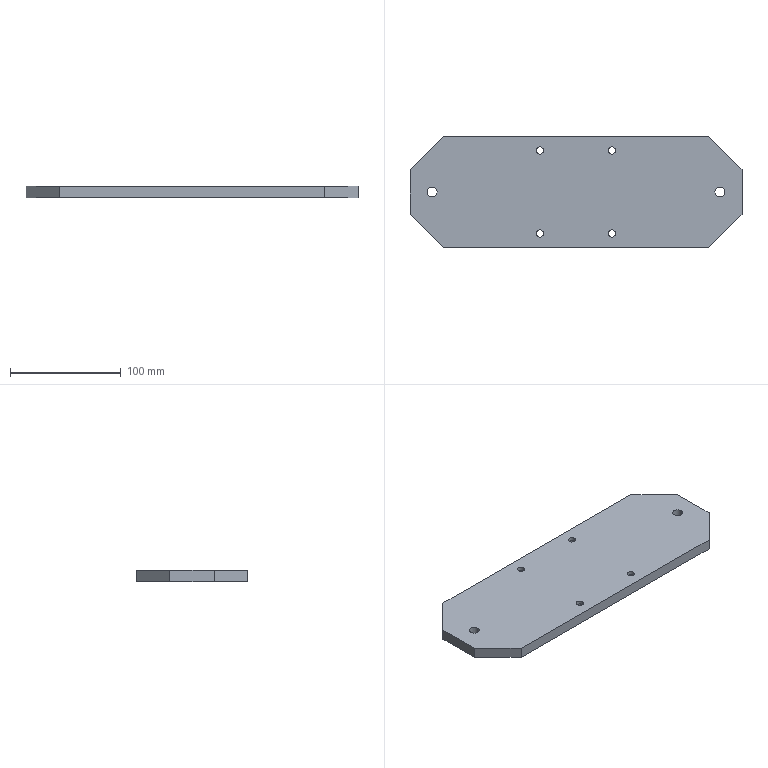Part | SolidWorks | features HoleWzd 2, Chamfer 1, Extrusion 1 | 1 solid | 34 faces | box 300 x 100 x 10 mm | volume 277705 mm3 | cylinder 20 | plane 14 | commonest cylinder face diameters 6.6 x8 11 x8 9 x4
STEP:
#1=CARTESIAN_POINT('',(125.5,0.,10.));
#2=VERTEX_POINT('',#1);
#3=CARTESIAN_POINT('',(134.5,0.,10.));
#4=VERTEX_POINT('',#3);
#5=CARTESIAN_POINT('',(130.,0.,10.));
#6=DIRECTION('',(0.,0.,1.));
#7=DIRECTION('',(1.,0.,0.));
#8=AXIS2_PLACEMENT_3D('',#5,#6,#7);
#9=CIRCLE('',#8,4.5);
#10=EDGE_CURVE('',#2,#4,#9,.T.);
#11=ORIENTED_EDGE('',*,*,#10,.T.);
#12=CARTESIAN_POINT('',(134.5,0.,0.));
#13=VERTEX_POINT('',#12);
#14=CARTESIAN_POINT('',(134.5,0.,0.));
#15=DIRECTION('',(0.,0.,-1.));
#16=VECTOR('',#15,1000.);
#17=LINE('',#14,#16);
#18=EDGE_CURVE('',#4,#13,#17,.T.);
#19=ORIENTED_EDGE('',*,*,#18,.T.);
#20=CARTESIAN_POINT('',(125.5,0.,0.));
#21=VERTEX_POINT('',#20);
#22=CARTESIAN_POINT('',(130.,0.,0.));
#23=DIRECTION('',(0.,0.,-1.));
#24=DIRECTION('',(-1.,0.,0.));
#25=AXIS2_PLACEMENT_3D('',#22,#23,#24);
#26=CIRCLE('',#25,4.5);
#27=EDGE_CURVE('',#13,#21,#26,.T.);
#28=ORIENTED_EDGE('',*,*,#27,.T.);
#29=CARTESIAN_POINT('',(125.5,0.,0.));
#30=DIRECTION('',(0.,0.,-1.));
#31=VECTOR('',#30,1000.);
#32=LINE('',#29,#31);
#33=EDGE_CURVE('',#2,#21,#32,.T.);
#34=ORIENTED_EDGE('',*,*,#33,.F.);
#35=EDGE_LOOP('',(#11,#19,#28,#34));
#36=FACE_OUTER_BOUND('',#35,.T.);
#37=CARTESIAN_POINT('',(130.,0.,0.));
#38=DIRECTION('',(0.,0.,-1.));
#39=DIRECTION('',(-1.,0.,0.));
#40=AXIS2_PLACEMENT_3D('',#37,#38,#39);
#41=CYLINDRICAL_SURFACE('',#40,4.5);
#42=ADVANCED_FACE('',(#36),#41,.F.);
#43=CARTESIAN_POINT('',(-134.5,0.,10.));
#44=VERTEX_POINT('',#43);
#45=CARTESIAN_POINT('',(-125.5,0.,10.));
#46=VERTEX_POINT('',#45);
#47=CARTESIAN_POINT('',(-130.,0.,10.));
#48=DIRECTION('',(0.,0.,1.));
#49=DIRECTION('',(1.,0.,0.));
#50=AXIS2_PLACEMENT_3D('',#47,#48,#49);
#51=CIRCLE('',#50,4.5);
#52=EDGE_CURVE('',#44,#46,#51,.T.);
#53=ORIENTED_EDGE('',*,*,#52,.T.);
#54=CARTESIAN_POINT('',(-125.5,0.,0.));
#55=VERTEX_POINT('',#54);
#56=CARTESIAN_POINT('',(-125.5,0.,0.));
#57=DIRECTION('',(0.,0.,-1.));
#58=VECTOR('',#57,1000.);
#59=LINE('',#56,#58);
#60=EDGE_CURVE('',#46,#55,#59,.T.);
#61=ORIENTED_EDGE('',*,*,#60,.T.);
#62=CARTESIAN_POINT('',(-134.5,0.,0.));
#63=VERTEX_POINT('',#62);
#64=CARTESIAN_POINT('',(-130.,0.,0.));
#65=DIRECTION('',(0.,0.,-1.));
#66=DIRECTION('',(-1.,0.,0.));
#67=AXIS2_PLACEMENT_3D('',#64,#65,#66);
#68=CIRCLE('',#67,4.5);
#69=EDGE_CURVE('',#55,#63,#68,.T.);
#70=ORIENTED_EDGE('',*,*,#69,.T.);
#71=CARTESIAN_POINT('',(-134.5,0.,0.));
#72=DIRECTION('',(0.,0.,-1.));
#73=VECTOR('',#72,1000.);
#74=LINE('',#71,#73);
#75=EDGE_CURVE('',#44,#63,#74,.T.);
#76=ORIENTED_EDGE('',*,*,#75,.F.);
#77=EDGE_LOOP('',(#53,#61,#70,#76));
#78=FACE_OUTER_BOUND('',#77,.T.);
#79=CARTESIAN_POINT('',(-130.,0.,0.));
#80=DIRECTION('',(0.,0.,-1.));
#81=DIRECTION('',(-1.,0.,0.));
#82=AXIS2_PLACEMENT_3D('',#79,#80,#81);
#83=CYLINDRICAL_SURFACE('',#82,4.5);
#84=ADVANCED_FACE('',(#78),#83,.F.);
#85=CARTESIAN_POINT('',(-27.1,-37.5,6.8));
#86=VERTEX_POINT('',#85);
#87=CARTESIAN_POINT('',(-38.1,-37.5,6.8));
#88=VERTEX_POINT('',#87);
#89=CARTESIAN_POINT('',(-32.6,-37.5,6.8));
#90=DIRECTION('',(0.,0.,-1.));
#91=DIRECTION('',(-1.,0.,0.));
#92=AXIS2_PLACEMENT_3D('',#89,#90,#91);
#93=CIRCLE('',#92,5.5);
#94=EDGE_CURVE('',#86,#88,#93,.T.);
#95=ORIENTED_EDGE('',*,*,#94,.F.);
#96=CARTESIAN_POINT('',(-27.1,-37.5,0.));
#97=VERTEX_POINT('',#96);
#98=CARTESIAN_POINT('',(-27.1,-37.5,0.));
#99=DIRECTION('',(0.,0.,-1.));
#100=VECTOR('',#99,1000.);
#101=LINE('',#98,#100);
#102=EDGE_CURVE('',#86,#97,#101,.T.);
#103=ORIENTED_EDGE('',*,*,#102,.T.);
#104=CARTESIAN_POINT('',(-38.1,-37.5,0.));
#105=VERTEX_POINT('',#104);
#106=CARTESIAN_POINT('',(-32.6,-37.5,0.));
#107=DIRECTION('',(0.,0.,-1.));
#108=DIRECTION('',(-1.,0.,0.));
#109=AXIS2_PLACEMENT_3D('',#106,#107,#108);
#110=CIRCLE('',#109,5.5);
#111=EDGE_CURVE('',#97,#105,#110,.T.);
#112=ORIENTED_EDGE('',*,*,#111,.T.);
#113=CARTESIAN_POINT('',(-38.1,-37.5,0.));
#114=DIRECTION('',(0.,0.,-1.));
#115=VECTOR('',#114,1000.);
#116=LINE('',#113,#115);
#117=EDGE_CURVE('',#88,#105,#116,.T.);
#118=ORIENTED_EDGE('',*,*,#117,.F.);
#119=EDGE_LOOP('',(#95,#103,#112,#118));
#120=FACE_OUTER_BOUND('',#119,.T.);
#121=CARTESIAN_POINT('',(-32.6,-37.5,0.));
#122=DIRECTION('',(0.,0.,-1.));
#123=DIRECTION('',(-1.,0.,0.));
#124=AXIS2_PLACEMENT_3D('',#121,#122,#123);
#125=CYLINDRICAL_SURFACE('',#124,5.5);
#126=ADVANCED_FACE('',(#120),#125,.F.);
#127=CARTESIAN_POINT('',(-35.9,-37.5,10.));
#128=VERTEX_POINT('',#127);
#129=CARTESIAN_POINT('',(-29.3,-37.5,10.));
#130=VERTEX_POINT('',#129);
#131=CARTESIAN_POINT('',(-32.6,-37.5,10.));
#132=DIRECTION('',(0.,0.,1.));
#133=DIRECTION('',(1.,0.,0.));
#134=AXIS2_PLACEMENT_3D('',#131,#132,#133);
#135=CIRCLE('',#134,3.3);
#136=EDGE_CURVE('',#128,#130,#135,.T.);
#137=ORIENTED_EDGE('',*,*,#136,.T.);
#138=CARTESIAN_POINT('',(-29.3,-37.5,6.8));
#139=VERTEX_POINT('',#138);
#140=CARTESIAN_POINT('',(-29.3,-37.5,0.));
#141=DIRECTION('',(0.,0.,-1.));
#142=VECTOR('',#141,1000.);
#143=LINE('',#140,#142);
#144=EDGE_CURVE('',#130,#139,#143,.T.);
#145=ORIENTED_EDGE('',*,*,#144,.T.);
#146=CARTESIAN_POINT('',(-35.9,-37.5,6.8));
#147=VERTEX_POINT('',#146);
#148=CARTESIAN_POINT('',(-32.6,-37.5,6.8));
#149=DIRECTION('',(0.,0.,-1.));
#150=DIRECTION('',(-1.,0.,0.));
#151=AXIS2_PLACEMENT_3D('',#148,#149,#150);
#152=CIRCLE('',#151,3.3);
#153=EDGE_CURVE('',#139,#147,#152,.T.);
#154=ORIENTED_EDGE('',*,*,#153,.T.);
#155=CARTESIAN_POINT('',(-35.9,-37.5,0.));
#156=DIRECTION('',(0.,0.,-1.));
#157=VECTOR('',#156,1000.);
#158=LINE('',#155,#157);
#159=EDGE_CURVE('',#128,#147,#158,.T.);
#160=ORIENTED_EDGE('',*,*,#159,.F.);
#161=EDGE_LOOP('',(#137,#145,#154,#160));
#162=FACE_OUTER_BOUND('',#161,.T.);
#163=CARTESIAN_POINT('',(-32.6,-37.5,0.));
#164=DIRECTION('',(0.,0.,-1.));
#165=DIRECTION('',(-1.,0.,0.));
#166=AXIS2_PLACEMENT_3D('',#163,#164,#165);
#167=CYLINDRICAL_SURFACE('',#166,3.3);
#168=ADVANCED_FACE('',(#162),#167,.F.);
#169=CARTESIAN_POINT('',(37.9,-37.5,6.8));
#170=VERTEX_POINT('',#169);
#171=CARTESIAN_POINT('',(26.9,-37.5,6.8));
#172=VERTEX_POINT('',#171);
#173=CARTESIAN_POINT('',(32.4,-37.5,6.8));
#174=DIRECTION('',(0.,0.,-1.));
#175=DIRECTION('',(-1.,0.,0.));
#176=AXIS2_PLACEMENT_3D('',#173,#174,#175);
#177=CIRCLE('',#176,5.5);
#178=EDGE_CURVE('',#170,#172,#177,.T.);
#179=ORIENTED_EDGE('',*,*,#178,.F.);
#180=CARTESIAN_POINT('',(37.9,-37.5,0.));
#181=VERTEX_POINT('',#180);
#182=CARTESIAN_POINT('',(37.9,-37.5,0.));
#183=DIRECTION('',(0.,0.,-1.));
#184=VECTOR('',#183,1000.);
#185=LINE('',#182,#184);
#186=EDGE_CURVE('',#170,#181,#185,.T.);
#187=ORIENTED_EDGE('',*,*,#186,.T.);
#188=CARTESIAN_POINT('',(26.9,-37.5,0.));
#189=VERTEX_POINT('',#188);
#190=CARTESIAN_POINT('',(32.4,-37.5,0.));
#191=DIRECTION('',(0.,0.,-1.));
#192=DIRECTION('',(-1.,0.,0.));
#193=AXIS2_PLACEMENT_3D('',#190,#191,#192);
#194=CIRCLE('',#193,5.5);
#195=EDGE_CURVE('',#181,#189,#194,.T.);
#196=ORIENTED_EDGE('',*,*,#195,.T.);
#197=CARTESIAN_POINT('',(26.9,-37.5,0.));
#198=DIRECTION('',(0.,0.,-1.));
#199=VECTOR('',#198,1000.);
#200=LINE('',#197,#199);
#201=EDGE_CURVE('',#172,#189,#200,.T.);
#202=ORIENTED_EDGE('',*,*,#201,.F.);
#203=EDGE_LOOP('',(#179,#187,#196,#202));
#204=FACE_OUTER_BOUND('',#203,.T.);
#205=CARTESIAN_POINT('',(32.4,-37.5,0.));
#206=DIRECTION('',(0.,0.,-1.));
#207=DIRECTION('',(-1.,0.,0.));
#208=AXIS2_PLACEMENT_3D('',#205,#206,#207);
#209=CYLINDRICAL_SURFACE('',#208,5.5);
#210=ADVANCED_FACE('',(#204),#209,.F.);
#211=CARTESIAN_POINT('',(29.1,-37.5,10.));
#212=VERTEX_POINT('',#211);
#213=CARTESIAN_POINT('',(35.7,-37.5,10.));
#214=VERTEX_POINT('',#213);
#215=CARTESIAN_POINT('',(32.4,-37.5,10.));
#216=DIRECTION('',(0.,0.,1.));
#217=DIRECTION('',(1.,0.,0.));
#218=AXIS2_PLACEMENT_3D('',#215,#216,#217);
#219=CIRCLE('',#218,3.3);
#220=EDGE_CURVE('',#212,#214,#219,.T.);
#221=ORIENTED_EDGE('',*,*,#220,.T.);
#222=CARTESIAN_POINT('',(35.7,-37.5,6.8));
#223=VERTEX_POINT('',#222);
#224=CARTESIAN_POINT('',(35.7,-37.5,0.));
#225=DIRECTION('',(0.,0.,-1.));
#226=VECTOR('',#225,1000.);
#227=LINE('',#224,#226);
#228=EDGE_CURVE('',#214,#223,#227,.T.);
#229=ORIENTED_EDGE('',*,*,#228,.T.);
#230=CARTESIAN_POINT('',(29.1,-37.5,6.8));
#231=VERTEX_POINT('',#230);
#232=CARTESIAN_POINT('',(32.4,-37.5,6.8));
#233=DIRECTION('',(0.,0.,-1.));
#234=DIRECTION('',(-1.,0.,0.));
#235=AXIS2_PLACEMENT_3D('',#232,#233,#234);
#236=CIRCLE('',#235,3.3);
#237=EDGE_CURVE('',#223,#231,#236,.T.);
#238=ORIENTED_EDGE('',*,*,#237,.T.);
#239=CARTESIAN_POINT('',(29.1,-37.5,0.));
#240=DIRECTION('',(0.,0.,-1.));
#241=VECTOR('',#240,1000.);
#242=LINE('',#239,#241);
#243=EDGE_CURVE('',#212,#231,#242,.T.);
#244=ORIENTED_EDGE('',*,*,#243,.F.);
#245=EDGE_LOOP('',(#221,#229,#238,#244));
#246=FACE_OUTER_BOUND('',#245,.T.);
#247=CARTESIAN_POINT('',(32.4,-37.5,0.));
#248=DIRECTION('',(0.,0.,-1.));
#249=DIRECTION('',(-1.,0.,0.));
#250=AXIS2_PLACEMENT_3D('',#247,#248,#249);
#251=CYLINDRICAL_SURFACE('',#250,3.3);
#252=ADVANCED_FACE('',(#246),#251,.F.);
#253=CARTESIAN_POINT('',(37.9,37.5,6.8));
#254=VERTEX_POINT('',#253);
#255=CARTESIAN_POINT('',(26.9,37.5,6.8));
#256=VERTEX_POINT('',#255);
#257=CARTESIAN_POINT('',(32.4,37.5,6.8));
#258=DIRECTION('',(0.,0.,-1.));
#259=DIRECTION('',(-1.,0.,0.));
#260=AXIS2_PLACEMENT_3D('',#257,#258,#259);
#261=CIRCLE('',#260,5.5);
#262=EDGE_CURVE('',#254,#256,#261,.T.);
#263=ORIENTED_EDGE('',*,*,#262,.F.);
#264=CARTESIAN_POINT('',(37.9,37.5,0.));
#265=VERTEX_POINT('',#264);
#266=CARTESIAN_POINT('',(37.9,37.5,0.));
#267=DIRECTION('',(0.,0.,-1.));
#268=VECTOR('',#267,1000.);
#269=LINE('',#266,#268);
#270=EDGE_CURVE('',#254,#265,#269,.T.);
#271=ORIENTED_EDGE('',*,*,#270,.T.);
#272=CARTESIAN_POINT('',(26.9,37.5,0.));
#273=VERTEX_POINT('',#272);
#274=CARTESIAN_POINT('',(32.4,37.5,0.));
#275=DIRECTION('',(0.,0.,-1.));
#276=DIRECTION('',(-1.,0.,0.));
#277=AXIS2_PLACEMENT_3D('',#274,#275,#276);
#278=CIRCLE('',#277,5.5);
#279=EDGE_CURVE('',#265,#273,#278,.T.);
#280=ORIENTED_EDGE('',*,*,#279,.T.);
#281=CARTESIAN_POINT('',(26.9,37.5,0.));
#282=DIRECTION('',(0.,0.,-1.));
#283=VECTOR('',#282,1000.);
#284=LINE('',#281,#283);
#285=EDGE_CURVE('',#256,#273,#284,.T.);
#286=ORIENTED_EDGE('',*,*,#285,.F.);
#287=EDGE_LOOP('',(#263,#271,#280,#286));
#288=FACE_OUTER_BOUND('',#287,.T.);
#289=CARTESIAN_POINT('',(32.4,37.5,0.));
#290=DIRECTION('',(0.,0.,-1.));
#291=DIRECTION('',(-1.,0.,0.));
#292=AXIS2_PLACEMENT_3D('',#289,#290,#291);
#293=CYLINDRICAL_SURFACE('',#292,5.5);
#294=ADVANCED_FACE('',(#288),#293,.F.);
#295=CARTESIAN_POINT('',(29.1,37.5,10.));
#296=VERTEX_POINT('',#295);
#297=CARTESIAN_POINT('',(35.7,37.5,10.));
#298=VERTEX_POINT('',#297);
#299=CARTESIAN_POINT('',(32.4,37.5,10.));
#300=DIRECTION('',(0.,0.,1.));
#301=DIRECTION('',(1.,0.,0.));
#302=AXIS2_PLACEMENT_3D('',#299,#300,#301);
#303=CIRCLE('',#302,3.3);
#304=EDGE_CURVE('',#296,#298,#303,.T.);
#305=ORIENTED_EDGE('',*,*,#304,.T.);
#306=CARTESIAN_POINT('',(35.7,37.5,6.8));
#307=VERTEX_POINT('',#306);
#308=CARTESIAN_POINT('',(35.7,37.5,0.));
#309=DIRECTION('',(0.,0.,-1.));
#310=VECTOR('',#309,1000.);
#311=LINE('',#308,#310);
#312=EDGE_CURVE('',#298,#307,#311,.T.);
#313=ORIENTED_EDGE('',*,*,#312,.T.);
#314=CARTESIAN_POINT('',(29.1,37.5,6.8));
#315=VERTEX_POINT('',#314);
#316=CARTESIAN_POINT('',(32.4,37.5,6.8));
#317=DIRECTION('',(0.,0.,-1.));
#318=DIRECTION('',(-1.,0.,0.));
#319=AXIS2_PLACEMENT_3D('',#316,#317,#318);
#320=CIRCLE('',#319,3.3);
#321=EDGE_CURVE('',#307,#315,#320,.T.);
#322=ORIENTED_EDGE('',*,*,#321,.T.);
#323=CARTESIAN_POINT('',(29.1,37.5,0.));
#324=DIRECTION('',(0.,0.,-1.));
#325=VECTOR('',#324,1000.);
#326=LINE('',#323,#325);
#327=EDGE_CURVE('',#296,#315,#326,.T.);
#328=ORIENTED_EDGE('',*,*,#327,.F.);
#329=EDGE_LOOP('',(#305,#313,#322,#328));
#330=FACE_OUTER_BOUND('',#329,.T.);
#331=CARTESIAN_POINT('',(32.4,37.5,0.));
#332=DIRECTION('',(0.,0.,-1.));
#333=DIRECTION('',(-1.,0.,0.));
#334=AXIS2_PLACEMENT_3D('',#331,#332,#333);
#335=CYLINDRICAL_SURFACE('',#334,3.3);
#336=ADVANCED_FACE('',(#330),#335,.F.);
#337=CARTESIAN_POINT('',(-27.1,37.5,6.8));
#338=VERTEX_POINT('',#337);
#339=CARTESIAN_POINT('',(-38.1,37.5,6.8));
#340=VERTEX_POINT('',#339);
#341=CARTESIAN_POINT('',(-32.6,37.5,6.8));
#342=DIRECTION('',(0.,0.,-1.));
#343=DIRECTION('',(-1.,0.,0.));
#344=AXIS2_PLACEMENT_3D('',#341,#342,#343);
#345=CIRCLE('',#344,5.5);
#346=EDGE_CURVE('',#338,#340,#345,.T.);
#347=ORIENTED_EDGE('',*,*,#346,.F.);
#348=CARTESIAN_POINT('',(-27.1,37.5,0.));
#349=VERTEX_POINT('',#348);
#350=CARTESIAN_POINT('',(-27.1,37.5,0.));
#351=DIRECTION('',(0.,0.,-1.));
#352=VECTOR('',#351,1000.);
#353=LINE('',#350,#352);
#354=EDGE_CURVE('',#338,#349,#353,.T.);
#355=ORIENTED_EDGE('',*,*,#354,.T.);
#356=CARTESIAN_POINT('',(-38.1,37.5,0.));
#357=VERTEX_POINT('',#356);
#358=CARTESIAN_POINT('',(-32.6,37.5,0.));
#359=DIRECTION('',(0.,0.,-1.));
#360=DIRECTION('',(-1.,0.,0.));
#361=AXIS2_PLACEMENT_3D('',#358,#359,#360);
#362=CIRCLE('',#361,5.5);
#363=EDGE_CURVE('',#349,#357,#362,.T.);
#364=ORIENTED_EDGE('',*,*,#363,.T.);
#365=CARTESIAN_POINT('',(-38.1,37.5,0.));
#366=DIRECTION('',(0.,0.,-1.));
#367=VECTOR('',#366,1000.);
#368=LINE('',#365,#367);
#369=EDGE_CURVE('',#340,#357,#368,.T.);
#370=ORIENTED_EDGE('',*,*,#369,.F.);
#371=EDGE_LOOP('',(#347,#355,#364,#370));
#372=FACE_OUTER_BOUND('',#371,.T.);
#373=CARTESIAN_POINT('',(-32.6,37.5,0.));
#374=DIRECTION('',(0.,0.,-1.));
#375=DIRECTION('',(-1.,0.,0.));
#376=AXIS2_PLACEMENT_3D('',#373,#374,#375);
#377=CYLINDRICAL_SURFACE('',#376,5.5);
#378=ADVANCED_FACE('',(#372),#377,.F.);
#379=CARTESIAN_POINT('',(-35.9,37.5,10.));
#380=VERTEX_POINT('',#379);
#381=CARTESIAN_POINT('',(-29.3,37.5,10.));
#382=VERTEX_POINT('',#381);
#383=CARTESIAN_POINT('',(-32.6,37.5,10.));
#384=DIRECTION('',(0.,0.,1.));
#385=DIRECTION('',(1.,0.,0.));
#386=AXIS2_PLACEMENT_3D('',#383,#384,#385);
#387=CIRCLE('',#386,3.3);
#388=EDGE_CURVE('',#380,#382,#387,.T.);
#389=ORIENTED_EDGE('',*,*,#388,.T.);
#390=CARTESIAN_POINT('',(-29.3,37.5,6.8));
#391=VERTEX_POINT('',#390);
#392=CARTESIAN_POINT('',(-29.3,37.5,0.));
#393=DIRECTION('',(0.,0.,-1.));
#394=VECTOR('',#393,1000.);
#395=LINE('',#392,#394);
#396=EDGE_CURVE('',#382,#391,#395,.T.);
#397=ORIENTED_EDGE('',*,*,#396,.T.);
#398=CARTESIAN_POINT('',(-35.9,37.5,6.8));
#399=VERTEX_POINT('',#398);
#400=CARTESIAN_POINT('',(-32.6,37.5,6.8));
#401=DIRECTION('',(0.,0.,-1.));
#402=DIRECTION('',(-1.,0.,0.));
#403=AXIS2_PLACEMENT_3D('',#400,#401,#402);
#404=CIRCLE('',#403,3.3);
#405=EDGE_CURVE('',#391,#399,#404,.T.);
#406=ORIENTED_EDGE('',*,*,#405,.T.);
#407=CARTESIAN_POINT('',(-35.9,37.5,0.));
#408=DIRECTION('',(0.,0.,-1.));
#409=VECTOR('',#408,1000.);
#410=LINE('',#407,#409);
#411=EDGE_CURVE('',#380,#399,#410,.T.);
#412=ORIENTED_EDGE('',*,*,#411,.F.);
#413=EDGE_LOOP('',(#389,#397,#406,#412));
#414=FACE_OUTER_BOUND('',#413,.T.);
#415=CARTESIAN_POINT('',(-32.6,37.5,0.));
#416=DIRECTION('',(0.,0.,-1.));
#417=DIRECTION('',(-1.,0.,0.));
#418=AXIS2_PLACEMENT_3D('',#415,#416,#417);
#419=CYLINDRICAL_SURFACE('',#418,3.3);
#420=ADVANCED_FACE('',(#414),#419,.F.);
#421=CARTESIAN_POINT('',(130.,0.,0.));
#422=DIRECTION('',(0.,0.,-1.));
#423=DIRECTION('',(-1.,0.,0.));
#424=AXIS2_PLACEMENT_3D('',#421,#422,#423);
#425=CIRCLE('',#424,4.5);
#426=EDGE_CURVE('',#21,#13,#425,.T.);
#427=ORIENTED_EDGE('',*,*,#426,.F.);
#428=ORIENTED_EDGE('',*,*,#27,.F.);
#429=EDGE_LOOP('',(#427,#428));
#430=FACE_BOUND('',#429,.T.);
#431=CARTESIAN_POINT('',(-32.6,-37.5,0.));
#432=DIRECTION('',(0.,0.,-1.));
#433=DIRECTION('',(-1.,0.,0.));
#434=AXIS2_PLACEMENT_3D('',#431,#432,#433);
#435=CIRCLE('',#434,5.5);
#436=EDGE_CURVE('',#105,#97,#435,.T.);
#437=ORIENTED_EDGE('',*,*,#436,.F.);
#438=ORIENTED_EDGE('',*,*,#111,.F.);
#439=EDGE_LOOP('',(#437,#438));
#440=FACE_BOUND('',#439,.T.);
#441=CARTESIAN_POINT('',(32.4,-37.5,0.));
#442=DIRECTION('',(0.,0.,-1.));
#443=DIRECTION('',(-1.,0.,0.));
#444=AXIS2_PLACEMENT_3D('',#441,#442,#443);
#445=CIRCLE('',#444,5.5);
#446=EDGE_CURVE('',#189,#181,#445,.T.);
#447=ORIENTED_EDGE('',*,*,#446,.F.);
#448=ORIENTED_EDGE('',*,*,#195,.F.);
#449=EDGE_LOOP('',(#447,#448));
#450=FACE_BOUND('',#449,.T.);
#451=CARTESIAN_POINT('',(32.4,37.5,0.));
#452=DIRECTION('',(0.,0.,-1.));
#453=DIRECTION('',(-1.,0.,0.));
#454=AXIS2_PLACEMENT_3D('',#451,#452,#453);
#455=CIRCLE('',#454,5.5);
#456=EDGE_CURVE('',#273,#265,#455,.T.);
#457=ORIENTED_EDGE('',*,*,#456,.F.);
#458=ORIENTED_EDGE('',*,*,#279,.F.);
#459=EDGE_LOOP('',(#457,#458));
#460=FACE_BOUND('',#459,.T.);
#461=CARTESIAN_POINT('',(-32.6,37.5,0.));
#462=DIRECTION('',(0.,0.,-1.));
#463=DIRECTION('',(-1.,0.,0.));
#464=AXIS2_PLACEMENT_3D('',#461,#462,#463);
#465=CIRCLE('',#464,5.5);
#466=EDGE_CURVE('',#357,#349,#465,.T.);
#467=ORIENTED_EDGE('',*,*,#466,.F.);
#468=ORIENTED_EDGE('',*,*,#363,.F.);
#469=EDGE_LOOP('',(#467,#468));
#470=FACE_BOUND('',#469,.T.);
#471=CARTESIAN_POINT('',(150.,-20.,0.));
#472=VERTEX_POINT('',#471);
#473=CARTESIAN_POINT('',(150.,20.,0.));
#474=VERTEX_POINT('',#473);
#475=CARTESIAN_POINT('',(150.,-50.,0.));
#476=DIRECTION('',(0.,1.,0.));
#477=VECTOR('',#476,1000.);
#478=LINE('',#475,#477);
#479=EDGE_CURVE('',#472,#474,#478,.T.);
#480=ORIENTED_EDGE('',*,*,#479,.F.);
#481=CARTESIAN_POINT('',(120.,-50.,0.));
#482=VERTEX_POINT('',#481);
#483=CARTESIAN_POINT('',(150.,-20.,0.));
#484=DIRECTION('',(-0.7071,-0.7071,0.));
#485=VECTOR('',#484,1000.);
#486=LINE('',#483,#485);
#487=EDGE_CURVE('',#472,#482,#486,.T.);
#488=ORIENTED_EDGE('',*,*,#487,.T.);
#489=CARTESIAN_POINT('',(-120.,-50.,0.));
#490=VERTEX_POINT('',#489);
#491=CARTESIAN_POINT('',(150.,-50.,0.));
#492=DIRECTION('',(1.,0.,0.));
#493=VECTOR('',#492,1000.);
#494=LINE('',#491,#493);
#495=EDGE_CURVE('',#490,#482,#494,.T.);
#496=ORIENTED_EDGE('',*,*,#495,.F.);
#497=CARTESIAN_POINT('',(-150.,-20.,0.));
#498=VERTEX_POINT('',#497);
#499=CARTESIAN_POINT('',(-120.,-50.,0.));
#500=DIRECTION('',(-0.7071,0.7071,0.));
#501=VECTOR('',#500,1000.);
#502=LINE('',#499,#501);
#503=EDGE_CURVE('',#490,#498,#502,.T.);
#504=ORIENTED_EDGE('',*,*,#503,.T.);
#505=CARTESIAN_POINT('',(-150.,20.,0.));
#506=VERTEX_POINT('',#505);
#507=CARTESIAN_POINT('',(-150.,-50.,0.));
#508=DIRECTION('',(0.,-1.,0.));
#509=VECTOR('',#508,1000.);
#510=LINE('',#507,#509);
#511=EDGE_CURVE('',#506,#498,#510,.T.);
#512=ORIENTED_EDGE('',*,*,#511,.F.);
#513=CARTESIAN_POINT('',(-120.,50.,0.));
#514=VERTEX_POINT('',#513);
#515=CARTESIAN_POINT('',(-150.,20.,0.));
#516=DIRECTION('',(0.7071,0.7071,0.));
#517=VECTOR('',#516,1000.);
#518=LINE('',#515,#517);
#519=EDGE_CURVE('',#506,#514,#518,.T.);
#520=ORIENTED_EDGE('',*,*,#519,.T.);
#521=CARTESIAN_POINT('',(120.,50.,0.));
#522=VERTEX_POINT('',#521);
#523=CARTESIAN_POINT('',(150.,50.,0.));
#524=DIRECTION('',(-1.,0.,0.));
#525=VECTOR('',#524,1000.);
#526=LINE('',#523,#525);
#527=EDGE_CURVE('',#522,#514,#526,.T.);
#528=ORIENTED_EDGE('',*,*,#527,.F.);
#529=CARTESIAN_POINT('',(120.,50.,0.));
#530=DIRECTION('',(0.7071,-0.7071,0.));
#531=VECTOR('',#530,1000.);
#532=LINE('',#529,#531);
#533=EDGE_CURVE('',#522,#474,#532,.T.);
#534=ORIENTED_EDGE('',*,*,#533,.T.);
#535=EDGE_LOOP('',(#480,#488,#496,#504,#512,#520,#528,#534));
#536=FACE_OUTER_BOUND('',#535,.T.);
#537=CARTESIAN_POINT('',(-130.,0.,0.));
#538=DIRECTION('',(0.,0.,-1.));
#539=DIRECTION('',(-1.,0.,0.));
#540=AXIS2_PLACEMENT_3D('',#537,#538,#539);
#541=CIRCLE('',#540,4.5);
#542=EDGE_CURVE('',#63,#55,#541,.T.);
#543=ORIENTED_EDGE('',*,*,#542,.F.);
#544=ORIENTED_EDGE('',*,*,#69,.F.);
#545=EDGE_LOOP('',(#543,#544));
#546=FACE_BOUND('',#545,.T.);
#547=CARTESIAN_POINT('',(0.,0.,0.));
#548=DIRECTION('',(0.,0.,1.));
#549=DIRECTION('',(1.,0.,0.));
#550=AXIS2_PLACEMENT_3D('',#547,#548,#549);
#551=PLANE('',#550);
#552=ADVANCED_FACE('',(#430,#440,#450,#460,#470,#536,#546),#551,.F.);
#553=CARTESIAN_POINT('',(-150.,20.,10.));
#554=VERTEX_POINT('',#553);
#555=CARTESIAN_POINT('',(-150.,-20.,10.));
#556=VERTEX_POINT('',#555);
#557=CARTESIAN_POINT('',(-150.,-50.,10.));
#558=DIRECTION('',(0.,-1.,0.));
#559=VECTOR('',#558,1000.);
#560=LINE('',#557,#559);
#561=EDGE_CURVE('',#554,#556,#560,.T.);
#562=ORIENTED_EDGE('',*,*,#561,.F.);
#563=CARTESIAN_POINT('',(-150.,20.,10.));
#564=DIRECTION('',(0.,0.,-1.));
#565=VECTOR('',#564,1000.);
#566=LINE('',#563,#565);
#567=EDGE_CURVE('',#554,#506,#566,.T.);
#568=ORIENTED_EDGE('',*,*,#567,.T.);
#569=ORIENTED_EDGE('',*,*,#511,.T.);
#570=CARTESIAN_POINT('',(-150.,-20.,10.));
#571=DIRECTION('',(0.,0.,1.));
#572=VECTOR('',#571,1000.);
#573=LINE('',#570,#572);
#574=EDGE_CURVE('',#498,#556,#573,.T.);
#575=ORIENTED_EDGE('',*,*,#574,.T.);
#576=EDGE_LOOP('',(#562,#568,#569,#575));
#577=FACE_OUTER_BOUND('',#576,.T.);
#578=CARTESIAN_POINT('',(-150.,-50.,10.));
#579=DIRECTION('',(1.,0.,0.));
#580=DIRECTION('',(0.,0.,-1.));
#581=AXIS2_PLACEMENT_3D('',#578,#579,#580);
#582=PLANE('',#581);
#583=ADVANCED_FACE('',(#577),#582,.F.);
#584=ORIENTED_EDGE('',*,*,#495,.T.);
#585=CARTESIAN_POINT('',(120.,-50.,10.));
#586=VERTEX_POINT('',#585);
#587=CARTESIAN_POINT('',(120.,-50.,10.));
#588=DIRECTION('',(0.,0.,1.));
#589=VECTOR('',#588,1000.);
#590=LINE('',#587,#589);
#591=EDGE_CURVE('',#482,#586,#590,.T.);
#592=ORIENTED_EDGE('',*,*,#591,.T.);
#593=CARTESIAN_POINT('',(-120.,-50.,10.));
#594=VERTEX_POINT('',#593);
#595=CARTESIAN_POINT('',(150.,-50.,10.));
#596=DIRECTION('',(1.,0.,0.));
#597=VECTOR('',#596,1000.);
#598=LINE('',#595,#597);
#599=EDGE_CURVE('',#594,#586,#598,.T.);
#600=ORIENTED_EDGE('',*,*,#599,.F.);
#601=CARTESIAN_POINT('',(-120.,-50.,10.));
#602=DIRECTION('',(0.,0.,-1.));
#603=VECTOR('',#602,1000.);
#604=LINE('',#601,#603);
#605=EDGE_CURVE('',#594,#490,#604,.T.);
#606=ORIENTED_EDGE('',*,*,#605,.T.);
#607=EDGE_LOOP('',(#584,#592,#600,#606));
#608=FACE_OUTER_BOUND('',#607,.T.);
#609=CARTESIAN_POINT('',(150.,-50.,10.));
#610=DIRECTION('',(0.,1.,0.));
#611=DIRECTION('',(-1.,0.,0.));
#612=AXIS2_PLACEMENT_3D('',#609,#610,#611);
#613=PLANE('',#612);
#614=ADVANCED_FACE('',(#608),#613,.F.);
#615=CARTESIAN_POINT('',(150.,-20.,10.));
#616=VERTEX_POINT('',#615);
#617=CARTESIAN_POINT('',(150.,20.,10.));
#618=VERTEX_POINT('',#617);
#619=CARTESIAN_POINT('',(150.,-50.,10.));
#620=DIRECTION('',(0.,1.,0.));
#621=VECTOR('',#620,1000.);
#622=LINE('',#619,#621);
#623=EDGE_CURVE('',#616,#618,#622,.T.);
#624=ORIENTED_EDGE('',*,*,#623,.F.);
#625=CARTESIAN_POINT('',(150.,-20.,10.));
#626=DIRECTION('',(0.,0.,-1.));
#627=VECTOR('',#626,1000.);
#628=LINE('',#625,#627);
#629=EDGE_CURVE('',#616,#472,#628,.T.);
#630=ORIENTED_EDGE('',*,*,#629,.T.);
#631=ORIENTED_EDGE('',*,*,#479,.T.);
#632=CARTESIAN_POINT('',(150.,20.,10.));
#633=DIRECTION('',(0.,0.,1.));
#634=VECTOR('',#633,1000.);
#635=LINE('',#632,#634);
#636=EDGE_CURVE('',#474,#618,#635,.T.);
#637=ORIENTED_EDGE('',*,*,#636,.T.);
#638=EDGE_LOOP('',(#624,#630,#631,#637));
#639=FACE_OUTER_BOUND('',#638,.T.);
#640=CARTESIAN_POINT('',(150.,-50.,10.));
#641=DIRECTION('',(-1.,0.,0.));
#642=DIRECTION('',(0.,0.,1.));
#643=AXIS2_PLACEMENT_3D('',#640,#641,#642);
#644=PLANE('',#643);
#645=ADVANCED_FACE('',(#639),#644,.F.);
#646=CARTESIAN_POINT('',(120.,50.,10.));
#647=VERTEX_POINT('',#646);
#648=CARTESIAN_POINT('',(-120.,50.,10.));
#649=VERTEX_POINT('',#648);
#650=CARTESIAN_POINT('',(150.,50.,10.));
#651=DIRECTION('',(-1.,0.,0.));
#652=VECTOR('',#651,1000.);
#653=LINE('',#650,#652);
#654=EDGE_CURVE('',#647,#649,#653,.T.);
#655=ORIENTED_EDGE('',*,*,#654,.F.);
#656=CARTESIAN_POINT('',(120.,50.,10.));
#657=DIRECTION('',(0.,0.,-1.));
#658=VECTOR('',#657,1000.);
#659=LINE('',#656,#658);
#660=EDGE_CURVE('',#647,#522,#659,.T.);
#661=ORIENTED_EDGE('',*,*,#660,.T.);
#662=ORIENTED_EDGE('',*,*,#527,.T.);
#663=CARTESIAN_POINT('',(-120.,50.,10.));
#664=DIRECTION('',(0.,0.,1.));
#665=VECTOR('',#664,1000.);
#666=LINE('',#663,#665);
#667=EDGE_CURVE('',#514,#649,#666,.T.);
#668=ORIENTED_EDGE('',*,*,#667,.T.);
#669=EDGE_LOOP('',(#655,#661,#662,#668));
#670=FACE_OUTER_BOUND('',#669,.T.);
#671=CARTESIAN_POINT('',(150.,50.,10.));
#672=DIRECTION('',(0.,-1.,0.));
#673=DIRECTION('',(1.,0.,0.));
#674=AXIS2_PLACEMENT_3D('',#671,#672,#673);
#675=PLANE('',#674);
#676=ADVANCED_FACE('',(#670),#675,.F.);
#677=ORIENTED_EDGE('',*,*,#10,.F.);
#678=CARTESIAN_POINT('',(130.,0.,10.));
#679=DIRECTION('',(0.,0.,1.));
#680=DIRECTION('',(1.,0.,0.));
#681=AXIS2_PLACEMENT_3D('',#678,#679,#680);
#682=CIRCLE('',#681,4.5);
#683=EDGE_CURVE('',#4,#2,#682,.T.);
#684=ORIENTED_EDGE('',*,*,#683,.F.);
#685=EDGE_LOOP('',(#677,#684));
#686=FACE_BOUND('',#685,.T.);
#687=ORIENTED_EDGE('',*,*,#52,.F.);
#688=CARTESIAN_POINT('',(-130.,0.,10.));
#689=DIRECTION('',(0.,0.,1.));
#690=DIRECTION('',(1.,0.,0.));
#691=AXIS2_PLACEMENT_3D('',#688,#689,#690);
#692=CIRCLE('',#691,4.5);
#693=EDGE_CURVE('',#46,#44,#692,.T.);
#694=ORIENTED_EDGE('',*,*,#693,.F.);
#695=EDGE_LOOP('',(#687,#694));
#696=FACE_BOUND('',#695,.T.);
#697=ORIENTED_EDGE('',*,*,#136,.F.);
#698=CARTESIAN_POINT('',(-32.6,-37.5,10.));
#699=DIRECTION('',(0.,0.,1.));
#700=DIRECTION('',(1.,0.,0.));
#701=AXIS2_PLACEMENT_3D('',#698,#699,#700);
#702=CIRCLE('',#701,3.3);
#703=EDGE_CURVE('',#130,#128,#702,.T.);
#704=ORIENTED_EDGE('',*,*,#703,.F.);
#705=EDGE_LOOP('',(#697,#704));
#706=FACE_BOUND('',#705,.T.);
#707=ORIENTED_EDGE('',*,*,#220,.F.);
#708=CARTESIAN_POINT('',(32.4,-37.5,10.));
#709=DIRECTION('',(0.,0.,1.));
#710=DIRECTION('',(1.,0.,0.));
#711=AXIS2_PLACEMENT_3D('',#708,#709,#710);
#712=CIRCLE('',#711,3.3);
#713=EDGE_CURVE('',#214,#212,#712,.T.);
#714=ORIENTED_EDGE('',*,*,#713,.F.);
#715=EDGE_LOOP('',(#707,#714));
#716=FACE_BOUND('',#715,.T.);
#717=ORIENTED_EDGE('',*,*,#304,.F.);
#718=CARTESIAN_POINT('',(32.4,37.5,10.));
#719=DIRECTION('',(0.,0.,1.));
#720=DIRECTION('',(1.,0.,0.));
#721=AXIS2_PLACEMENT_3D('',#718,#719,#720);
#722=CIRCLE('',#721,3.3);
#723=EDGE_CURVE('',#298,#296,#722,.T.);
#724=ORIENTED_EDGE('',*,*,#723,.F.);
#725=EDGE_LOOP('',(#717,#724));
#726=FACE_BOUND('',#725,.T.);
#727=ORIENTED_EDGE('',*,*,#388,.F.);
#728=CARTESIAN_POINT('',(-32.6,37.5,10.));
#729=DIRECTION('',(0.,0.,1.));
#730=DIRECTION('',(1.,0.,0.));
#731=AXIS2_PLACEMENT_3D('',#728,#729,#730);
#732=CIRCLE('',#731,3.3);
#733=EDGE_CURVE('',#382,#380,#732,.T.);
#734=ORIENTED_EDGE('',*,*,#733,.F.);
#735=EDGE_LOOP('',(#727,#734));
#736=FACE_BOUND('',#735,.T.);
#737=ORIENTED_EDGE('',*,*,#599,.T.);
#738=CARTESIAN_POINT('',(85.,-85.,10.));
#739=DIRECTION('',(0.7071,0.7071,0.));
#740=VECTOR('',#739,1000.);
#741=LINE('',#738,#740);
#742=EDGE_CURVE('',#586,#616,#741,.T.);
#743=ORIENTED_EDGE('',*,*,#742,.T.);
#744=ORIENTED_EDGE('',*,*,#623,.T.);
#745=CARTESIAN_POINT('',(85.,85.,10.));
#746=DIRECTION('',(-0.7071,0.7071,0.));
#747=VECTOR('',#746,1000.);
#748=LINE('',#745,#747);
#749=EDGE_CURVE('',#618,#647,#748,.T.);
#750=ORIENTED_EDGE('',*,*,#749,.T.);
#751=ORIENTED_EDGE('',*,*,#654,.T.);
#752=CARTESIAN_POINT('',(-85.,85.,10.));
#753=DIRECTION('',(-0.7071,-0.7071,0.));
#754=VECTOR('',#753,1000.);
#755=LINE('',#752,#754);
#756=EDGE_CURVE('',#649,#554,#755,.T.);
#757=ORIENTED_EDGE('',*,*,#756,.T.);
#758=ORIENTED_EDGE('',*,*,#561,.T.);
#759=CARTESIAN_POINT('',(-85.,-85.,10.));
#760=DIRECTION('',(0.7071,-0.7071,0.));
#761=VECTOR('',#760,1000.);
#762=LINE('',#759,#761);
#763=EDGE_CURVE('',#556,#594,#762,.T.);
#764=ORIENTED_EDGE('',*,*,#763,.T.);
#765=EDGE_LOOP('',(#737,#743,#744,#750,#751,#757,#758,#764));
#766=FACE_OUTER_BOUND('',#765,.T.);
#767=CARTESIAN_POINT('',(0.,0.,10.));
#768=DIRECTION('',(0.,0.,1.));
#769=DIRECTION('',(1.,0.,0.));
#770=AXIS2_PLACEMENT_3D('',#767,#768,#769);
#771=PLANE('',#770);
#772=ADVANCED_FACE('',(#686,#696,#706,#716,#726,#736,#766),#771,.T.);
#773=ORIENTED_EDGE('',*,*,#396,.F.);
#774=ORIENTED_EDGE('',*,*,#733,.T.);
#775=ORIENTED_EDGE('',*,*,#411,.T.);
#776=CARTESIAN_POINT('',(-32.6,37.5,6.8));
#777=DIRECTION('',(0.,0.,-1.));
#778=DIRECTION('',(-1.,0.,0.));
#779=AXIS2_PLACEMENT_3D('',#776,#777,#778);
#780=CIRCLE('',#779,3.3);
#781=EDGE_CURVE('',#399,#391,#780,.T.);
#782=ORIENTED_EDGE('',*,*,#781,.T.);
#783=EDGE_LOOP('',(#773,#774,#775,#782));
#784=FACE_OUTER_BOUND('',#783,.T.);
#785=CARTESIAN_POINT('',(-32.6,37.5,0.));
#786=DIRECTION('',(0.,0.,-1.));
#787=DIRECTION('',(-1.,0.,0.));
#788=AXIS2_PLACEMENT_3D('',#785,#786,#787);
#789=CYLINDRICAL_SURFACE('',#788,3.3);
#790=ADVANCED_FACE('',(#784),#789,.F.);
#791=ORIENTED_EDGE('',*,*,#781,.F.);
#792=ORIENTED_EDGE('',*,*,#405,.F.);
#793=EDGE_LOOP('',(#791,#792));
#794=FACE_BOUND('',#793,.T.);
#795=CARTESIAN_POINT('',(-32.6,37.5,6.8));
#796=DIRECTION('',(0.,0.,-1.));
#797=DIRECTION('',(-1.,0.,0.));
#798=AXIS2_PLACEMENT_3D('',#795,#796,#797);
#799=CIRCLE('',#798,5.5);
#800=EDGE_CURVE('',#340,#338,#799,.T.);
#801=ORIENTED_EDGE('',*,*,#800,.T.);
#802=ORIENTED_EDGE('',*,*,#346,.T.);
#803=EDGE_LOOP('',(#801,#802));
#804=FACE_OUTER_BOUND('',#803,.T.);
#805=CARTESIAN_POINT('',(-29.3,37.5,6.8));
#806=DIRECTION('',(0.,0.,1.));
#807=DIRECTION('',(1.,0.,0.));
#808=AXIS2_PLACEMENT_3D('',#805,#806,#807);
#809=PLANE('',#808);
#810=ADVANCED_FACE('',(#794,#804),#809,.F.);
#811=ORIENTED_EDGE('',*,*,#354,.F.);
#812=ORIENTED_EDGE('',*,*,#800,.F.);
#813=ORIENTED_EDGE('',*,*,#369,.T.);
#814=ORIENTED_EDGE('',*,*,#466,.T.);
#815=EDGE_LOOP('',(#811,#812,#813,#814));
#816=FACE_OUTER_BOUND('',#815,.T.);
#817=CARTESIAN_POINT('',(-32.6,37.5,0.));
#818=DIRECTION('',(0.,0.,-1.));
#819=DIRECTION('',(-1.,0.,0.));
#820=AXIS2_PLACEMENT_3D('',#817,#818,#819);
#821=CYLINDRICAL_SURFACE('',#820,5.5);
#822=ADVANCED_FACE('',(#816),#821,.F.);
#823=ORIENTED_EDGE('',*,*,#312,.F.);
#824=ORIENTED_EDGE('',*,*,#723,.T.);
#825=ORIENTED_EDGE('',*,*,#327,.T.);
#826=CARTESIAN_POINT('',(32.4,37.5,6.8));
#827=DIRECTION('',(0.,0.,-1.));
#828=DIRECTION('',(-1.,0.,0.));
#829=AXIS2_PLACEMENT_3D('',#826,#827,#828);
#830=CIRCLE('',#829,3.3);
#831=EDGE_CURVE('',#315,#307,#830,.T.);
#832=ORIENTED_EDGE('',*,*,#831,.T.);
#833=EDGE_LOOP('',(#823,#824,#825,#832));
#834=FACE_OUTER_BOUND('',#833,.T.);
#835=CARTESIAN_POINT('',(32.4,37.5,0.));
#836=DIRECTION('',(0.,0.,-1.));
#837=DIRECTION('',(-1.,0.,0.));
#838=AXIS2_PLACEMENT_3D('',#835,#836,#837);
#839=CYLINDRICAL_SURFACE('',#838,3.3);
#840=ADVANCED_FACE('',(#834),#839,.F.);
#841=ORIENTED_EDGE('',*,*,#831,.F.);
#842=ORIENTED_EDGE('',*,*,#321,.F.);
#843=EDGE_LOOP('',(#841,#842));
#844=FACE_BOUND('',#843,.T.);
#845=CARTESIAN_POINT('',(32.4,37.5,6.8));
#846=DIRECTION('',(0.,0.,-1.));
#847=DIRECTION('',(-1.,0.,0.));
#848=AXIS2_PLACEMENT_3D('',#845,#846,#847);
#849=CIRCLE('',#848,5.5);
#850=EDGE_CURVE('',#256,#254,#849,.T.);
#851=ORIENTED_EDGE('',*,*,#850,.T.);
#852=ORIENTED_EDGE('',*,*,#262,.T.);
#853=EDGE_LOOP('',(#851,#852));
#854=FACE_OUTER_BOUND('',#853,.T.);
#855=CARTESIAN_POINT('',(35.7,37.5,6.8));
#856=DIRECTION('',(0.,0.,1.));
#857=DIRECTION('',(1.,0.,0.));
#858=AXIS2_PLACEMENT_3D('',#855,#856,#857);
#859=PLANE('',#858);
#860=ADVANCED_FACE('',(#844,#854),#859,.F.);
#861=ORIENTED_EDGE('',*,*,#270,.F.);
#862=ORIENTED_EDGE('',*,*,#850,.F.);
#863=ORIENTED_EDGE('',*,*,#285,.T.);
#864=ORIENTED_EDGE('',*,*,#456,.T.);
#865=EDGE_LOOP('',(#861,#862,#863,#864));
#866=FACE_OUTER_BOUND('',#865,.T.);
#867=CARTESIAN_POINT('',(32.4,37.5,0.));
#868=DIRECTION('',(0.,0.,-1.));
#869=DIRECTION('',(-1.,0.,0.));
#870=AXIS2_PLACEMENT_3D('',#867,#868,#869);
#871=CYLINDRICAL_SURFACE('',#870,5.5);
#872=ADVANCED_FACE('',(#866),#871,.F.);
#873=ORIENTED_EDGE('',*,*,#228,.F.);
#874=ORIENTED_EDGE('',*,*,#713,.T.);
#875=ORIENTED_EDGE('',*,*,#243,.T.);
#876=CARTESIAN_POINT('',(32.4,-37.5,6.8));
#877=DIRECTION('',(0.,0.,-1.));
#878=DIRECTION('',(-1.,0.,0.));
#879=AXIS2_PLACEMENT_3D('',#876,#877,#878);
#880=CIRCLE('',#879,3.3);
#881=EDGE_CURVE('',#231,#223,#880,.T.);
#882=ORIENTED_EDGE('',*,*,#881,.T.);
#883=EDGE_LOOP('',(#873,#874,#875,#882));
#884=FACE_OUTER_BOUND('',#883,.T.);
#885=CARTESIAN_POINT('',(32.4,-37.5,0.));
#886=DIRECTION('',(0.,0.,-1.));
#887=DIRECTION('',(-1.,0.,0.));
#888=AXIS2_PLACEMENT_3D('',#885,#886,#887);
#889=CYLINDRICAL_SURFACE('',#888,3.3);
#890=ADVANCED_FACE('',(#884),#889,.F.);
#891=ORIENTED_EDGE('',*,*,#881,.F.);
#892=ORIENTED_EDGE('',*,*,#237,.F.);
#893=EDGE_LOOP('',(#891,#892));
#894=FACE_BOUND('',#893,.T.);
#895=CARTESIAN_POINT('',(32.4,-37.5,6.8));
#896=DIRECTION('',(0.,0.,-1.));
#897=DIRECTION('',(-1.,0.,0.));
#898=AXIS2_PLACEMENT_3D('',#895,#896,#897);
#899=CIRCLE('',#898,5.5);
#900=EDGE_CURVE('',#172,#170,#899,.T.);
#901=ORIENTED_EDGE('',*,*,#900,.T.);
#902=ORIENTED_EDGE('',*,*,#178,.T.);
#903=EDGE_LOOP('',(#901,#902));
#904=FACE_OUTER_BOUND('',#903,.T.);
#905=CARTESIAN_POINT('',(35.7,-37.5,6.8));
#906=DIRECTION('',(0.,0.,1.));
#907=DIRECTION('',(1.,0.,0.));
#908=AXIS2_PLACEMENT_3D('',#905,#906,#907);
#909=PLANE('',#908);
#910=ADVANCED_FACE('',(#894,#904),#909,.F.);
#911=ORIENTED_EDGE('',*,*,#186,.F.);
#912=ORIENTED_EDGE('',*,*,#900,.F.);
#913=ORIENTED_EDGE('',*,*,#201,.T.);
#914=ORIENTED_EDGE('',*,*,#446,.T.);
#915=EDGE_LOOP('',(#911,#912,#913,#914));
#916=FACE_OUTER_BOUND('',#915,.T.);
#917=CARTESIAN_POINT('',(32.4,-37.5,0.));
#918=DIRECTION('',(0.,0.,-1.));
#919=DIRECTION('',(-1.,0.,0.));
#920=AXIS2_PLACEMENT_3D('',#917,#918,#919);
#921=CYLINDRICAL_SURFACE('',#920,5.5);
#922=ADVANCED_FACE('',(#916),#921,.F.);
#923=ORIENTED_EDGE('',*,*,#144,.F.);
#924=ORIENTED_EDGE('',*,*,#703,.T.);
#925=ORIENTED_EDGE('',*,*,#159,.T.);
#926=CARTESIAN_POINT('',(-32.6,-37.5,6.8));
#927=DIRECTION('',(0.,0.,-1.));
#928=DIRECTION('',(-1.,0.,0.));
#929=AXIS2_PLACEMENT_3D('',#926,#927,#928);
#930=CIRCLE('',#929,3.3);
#931=EDGE_CURVE('',#147,#139,#930,.T.);
#932=ORIENTED_EDGE('',*,*,#931,.T.);
#933=EDGE_LOOP('',(#923,#924,#925,#932));
#934=FACE_OUTER_BOUND('',#933,.T.);
#935=CARTESIAN_POINT('',(-32.6,-37.5,0.));
#936=DIRECTION('',(0.,0.,-1.));
#937=DIRECTION('',(-1.,0.,0.));
#938=AXIS2_PLACEMENT_3D('',#935,#936,#937);
#939=CYLINDRICAL_SURFACE('',#938,3.3);
#940=ADVANCED_FACE('',(#934),#939,.F.);
#941=ORIENTED_EDGE('',*,*,#931,.F.);
#942=ORIENTED_EDGE('',*,*,#153,.F.);
#943=EDGE_LOOP('',(#941,#942));
#944=FACE_BOUND('',#943,.T.);
#945=CARTESIAN_POINT('',(-32.6,-37.5,6.8));
#946=DIRECTION('',(0.,0.,-1.));
#947=DIRECTION('',(-1.,0.,0.));
#948=AXIS2_PLACEMENT_3D('',#945,#946,#947);
#949=CIRCLE('',#948,5.5);
#950=EDGE_CURVE('',#88,#86,#949,.T.);
#951=ORIENTED_EDGE('',*,*,#950,.T.);
#952=ORIENTED_EDGE('',*,*,#94,.T.);
#953=EDGE_LOOP('',(#951,#952));
#954=FACE_OUTER_BOUND('',#953,.T.);
#955=CARTESIAN_POINT('',(-29.3,-37.5,6.8));
#956=DIRECTION('',(0.,0.,1.));
#957=DIRECTION('',(1.,0.,0.));
#958=AXIS2_PLACEMENT_3D('',#955,#956,#957);
#959=PLANE('',#958);
#960=ADVANCED_FACE('',(#944,#954),#959,.F.);
#961=ORIENTED_EDGE('',*,*,#102,.F.);
#962=ORIENTED_EDGE('',*,*,#950,.F.);
#963=ORIENTED_EDGE('',*,*,#117,.T.);
#964=ORIENTED_EDGE('',*,*,#436,.T.);
#965=EDGE_LOOP('',(#961,#962,#963,#964));
#966=FACE_OUTER_BOUND('',#965,.T.);
#967=CARTESIAN_POINT('',(-32.6,-37.5,0.));
#968=DIRECTION('',(0.,0.,-1.));
#969=DIRECTION('',(-1.,0.,0.));
#970=AXIS2_PLACEMENT_3D('',#967,#968,#969);
#971=CYLINDRICAL_SURFACE('',#970,5.5);
#972=ADVANCED_FACE('',(#966),#971,.F.);
#973=ORIENTED_EDGE('',*,*,#60,.F.);
#974=ORIENTED_EDGE('',*,*,#693,.T.);
#975=ORIENTED_EDGE('',*,*,#75,.T.);
#976=ORIENTED_EDGE('',*,*,#542,.T.);
#977=EDGE_LOOP('',(#973,#974,#975,#976));
#978=FACE_OUTER_BOUND('',#977,.T.);
#979=CARTESIAN_POINT('',(-130.,0.,0.));
#980=DIRECTION('',(0.,0.,-1.));
#981=DIRECTION('',(-1.,0.,0.));
#982=AXIS2_PLACEMENT_3D('',#979,#980,#981);
#983=CYLINDRICAL_SURFACE('',#982,4.5);
#984=ADVANCED_FACE('',(#978),#983,.F.);
#985=ORIENTED_EDGE('',*,*,#18,.F.);
#986=ORIENTED_EDGE('',*,*,#683,.T.);
#987=ORIENTED_EDGE('',*,*,#33,.T.);
#988=ORIENTED_EDGE('',*,*,#426,.T.);
#989=EDGE_LOOP('',(#985,#986,#987,#988));
#990=FACE_OUTER_BOUND('',#989,.T.);
#991=CARTESIAN_POINT('',(130.,0.,0.));
#992=DIRECTION('',(0.,0.,-1.));
#993=DIRECTION('',(-1.,0.,0.));
#994=AXIS2_PLACEMENT_3D('',#991,#992,#993);
#995=CYLINDRICAL_SURFACE('',#994,4.5);
#996=ADVANCED_FACE('',(#990),#995,.F.);
#997=ORIENTED_EDGE('',*,*,#742,.F.);
#998=ORIENTED_EDGE('',*,*,#591,.F.);
#999=ORIENTED_EDGE('',*,*,#487,.F.);
#1000=ORIENTED_EDGE('',*,*,#629,.F.);
#1001=EDGE_LOOP('',(#997,#998,#999,#1000));
#1002=FACE_OUTER_BOUND('',#1001,.T.);
#1003=CARTESIAN_POINT('',(150.,-20.,10.));
#1004=DIRECTION('',(-0.7071,0.7071,0.));
#1005=DIRECTION('',(0.,0.,-1.));
#1006=AXIS2_PLACEMENT_3D('',#1003,#1004,#1005);
#1007=PLANE('',#1006);
#1008=ADVANCED_FACE('',(#1002),#1007,.F.);
#1009=ORIENTED_EDGE('',*,*,#749,.F.);
#1010=ORIENTED_EDGE('',*,*,#636,.F.);
#1011=ORIENTED_EDGE('',*,*,#533,.F.);
#1012=ORIENTED_EDGE('',*,*,#660,.F.);
#1013=EDGE_LOOP('',(#1009,#1010,#1011,#1012));
#1014=FACE_OUTER_BOUND('',#1013,.T.);
#1015=CARTESIAN_POINT('',(120.,50.,10.));
#1016=DIRECTION('',(-0.7071,-0.7071,0.));
#1017=DIRECTION('',(0.,0.,-1.));
#1018=AXIS2_PLACEMENT_3D('',#1015,#1016,#1017);
#1019=PLANE('',#1018);
#1020=ADVANCED_FACE('',(#1014),#1019,.F.);
#1021=ORIENTED_EDGE('',*,*,#756,.F.);
#1022=ORIENTED_EDGE('',*,*,#667,.F.);
#1023=ORIENTED_EDGE('',*,*,#519,.F.);
#1024=ORIENTED_EDGE('',*,*,#567,.F.);
#1025=EDGE_LOOP('',(#1021,#1022,#1023,#1024));
#1026=FACE_OUTER_BOUND('',#1025,.T.);
#1027=CARTESIAN_POINT('',(-150.,20.,10.));
#1028=DIRECTION('',(0.7071,-0.7071,0.));
#1029=DIRECTION('',(0.,0.,-1.));
#1030=AXIS2_PLACEMENT_3D('',#1027,#1028,#1029);
#1031=PLANE('',#1030);
#1032=ADVANCED_FACE('',(#1026),#1031,.F.);
#1033=ORIENTED_EDGE('',*,*,#763,.F.);
#1034=ORIENTED_EDGE('',*,*,#574,.F.);
#1035=ORIENTED_EDGE('',*,*,#503,.F.);
#1036=ORIENTED_EDGE('',*,*,#605,.F.);
#1037=EDGE_LOOP('',(#1033,#1034,#1035,#1036));
#1038=FACE_OUTER_BOUND('',#1037,.T.);
#1039=CARTESIAN_POINT('',(-120.,-50.,10.));
#1040=DIRECTION('',(0.7071,0.7071,0.));
#1041=DIRECTION('',(0.,0.,-1.));
#1042=AXIS2_PLACEMENT_3D('',#1039,#1040,#1041);
#1043=PLANE('',#1042);
#1044=ADVANCED_FACE('',(#1038),#1043,.F.);
#1045=CLOSED_SHELL('',(#42,#84,#126,#168,#210,#252,#294,#336,#378,#420,#552,#583,#614,#645,#676,#772,#790,#810,#822,#840,#860,#872,#890,#910,#922,#940,#960,#972,#984,#996,#1008,#1020,#1032,#1044));
#1046=MANIFOLD_SOLID_BREP('',#1045);
#1047=CARTESIAN_POINT('',(0.,0.,0.));
#1048=DIRECTION('',(0.,0.,1.));
#1049=DIRECTION('',(1.,0.,0.));
#1050=AXIS2_PLACEMENT_3D('',#1047,#1048,#1049);
#1051=(LENGTH_UNIT()NAMED_UNIT(*)SI_UNIT(.MILLI.,.METRE.));
#1052=UNCERTAINTY_MEASURE_WITH_UNIT(LENGTH_MEASURE(0.00001),#1051,'','');
#1053=(NAMED_UNIT(*)PLANE_ANGLE_UNIT()SI_UNIT($,.RADIAN.));
#1054=(NAMED_UNIT(*)SI_UNIT($,.STERADIAN.)SOLID_ANGLE_UNIT());
#1055=(GEOMETRIC_REPRESENTATION_CONTEXT(3)GLOBAL_UNCERTAINTY_ASSIGNED_CONTEXT((#1052))GLOBAL_UNIT_ASSIGNED_CONTEXT((#1051,#1053,#1054))REPRESENTATION_CONTEXT('',''));
#1056=ADVANCED_BREP_SHAPE_REPRESENTATION('',(#1046,#1050),#1055);